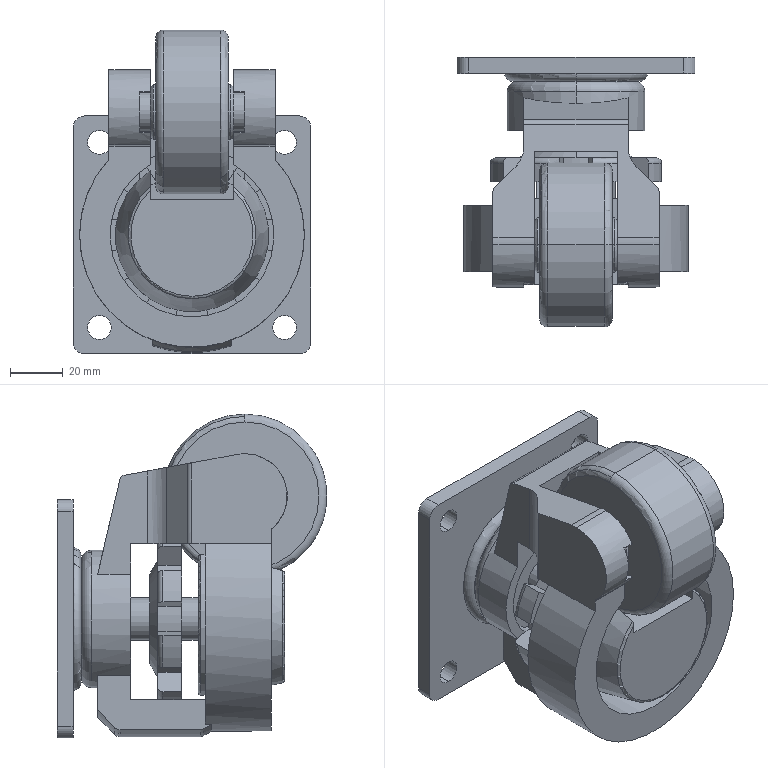Part | STEP file | 001-001-hcaaa-d80-nj | 1 solid | 201 faces | box 90 x 102 x 122.5 mm | volume 382378 mm3 | plane 85 | cylinder 80 | torus 24 | cone 12 | commonest cylinder face diameters 9 x12 66 x10 48.667 x9 16 x8 10.667 x5 62 x5